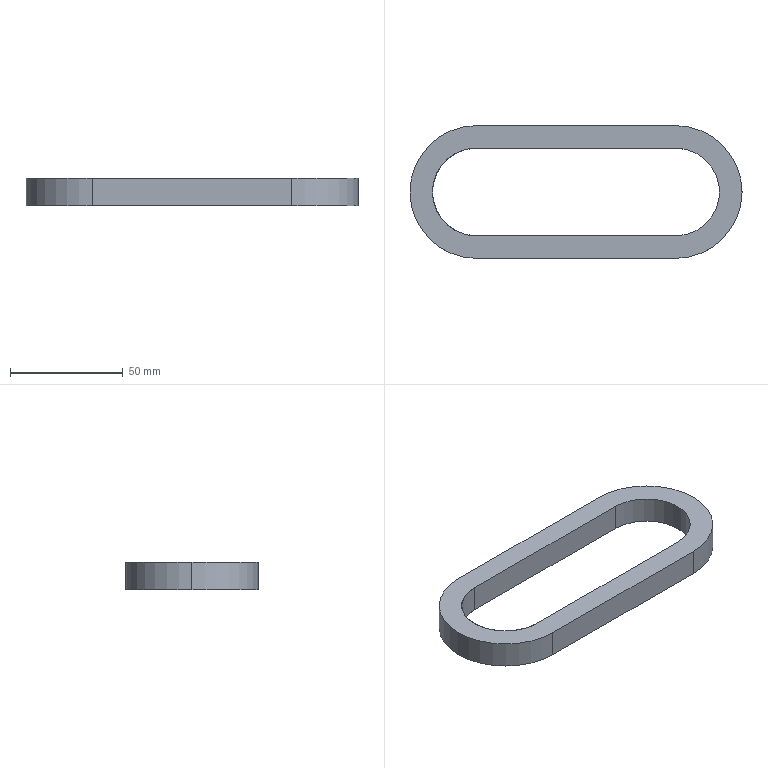Part | NX | features BREP 1, DATUM_CSYS 1, EXTRACT_DATUM_PLANE 1, EXTRUDE 1, SKETCH 1 | 2 solids | 22 faces | box 147.5 x 59 x 12 mm | volume 79425 mm3 | plane 12 | cylinder 10 | commonest cylinder face diameters 39 x5 59 x5
STEP:
#1=CARTESIAN_POINT('',(675.25,133.707,6.));
#2=VERTEX_POINT('',#1);
#3=CARTESIAN_POINT('',(675.25,133.707,-6.));
#4=VERTEX_POINT('',#3);
#5=CARTESIAN_POINT('',(675.25,133.707,6.));
#6=DIRECTION('',(0.,0.,-1.));
#7=VECTOR('',#6,1000.);
#8=LINE('',#5,#7);
#9=EDGE_CURVE('',#2,#4,#8,.T.);
#10=ORIENTED_EDGE('',*,*,#9,.F.);
#11=CARTESIAN_POINT('',(763.75,133.707,6.));
#12=VERTEX_POINT('',#11);
#13=CARTESIAN_POINT('',(675.25,133.707,6.));
#14=DIRECTION('',(1.,0.,0.));
#15=VECTOR('',#14,1000.);
#16=LINE('',#13,#15);
#17=EDGE_CURVE('',#2,#12,#16,.T.);
#18=ORIENTED_EDGE('',*,*,#17,.T.);
#19=CARTESIAN_POINT('',(763.75,133.707,-6.));
#20=VERTEX_POINT('',#19);
#21=CARTESIAN_POINT('',(763.75,133.707,-6.));
#22=DIRECTION('',(0.,0.,1.));
#23=VECTOR('',#22,1000.);
#24=LINE('',#21,#23);
#25=EDGE_CURVE('',#20,#12,#24,.T.);
#26=ORIENTED_EDGE('',*,*,#25,.F.);
#27=CARTESIAN_POINT('',(675.25,133.707,-6.));
#28=DIRECTION('',(1.,0.,0.));
#29=VECTOR('',#28,1000.);
#30=LINE('',#27,#29);
#31=EDGE_CURVE('',#4,#20,#30,.T.);
#32=ORIENTED_EDGE('',*,*,#31,.F.);
#33=EDGE_LOOP('',(#10,#18,#26,#32));
#34=FACE_BOUND('',#33,.T.);
#35=CARTESIAN_POINT('',(675.25,133.707,6.));
#36=DIRECTION('',(0.,-1.,0.));
#37=DIRECTION('',(0.,0.,1.));
#38=AXIS2_PLACEMENT_3D('',#35,#36,#37);
#39=PLANE('',#38);
#40=ADVANCED_FACE('',(#34),#39,.F.);
#41=ORIENTED_EDGE('',*,*,#31,.T.);
#42=CARTESIAN_POINT('',(763.75,74.707,-6.));
#43=VERTEX_POINT('',#42);
#44=CARTESIAN_POINT('',(763.75,104.207,-6.));
#45=DIRECTION('',(0.,0.,-1.));
#46=DIRECTION('',(0.,1.,0.));
#47=AXIS2_PLACEMENT_3D('',#44,#45,#46);
#48=CIRCLE('',#47,29.5);
#49=EDGE_CURVE('',#20,#43,#48,.T.);
#50=ORIENTED_EDGE('',*,*,#49,.T.);
#51=CARTESIAN_POINT('',(675.25,74.707,-6.));
#52=VERTEX_POINT('',#51);
#53=CARTESIAN_POINT('',(763.75,74.707,-6.));
#54=DIRECTION('',(-1.,0.,0.));
#55=VECTOR('',#54,1000.);
#56=LINE('',#53,#55);
#57=EDGE_CURVE('',#43,#52,#56,.T.);
#58=ORIENTED_EDGE('',*,*,#57,.T.);
#59=CARTESIAN_POINT('',(645.75,104.207,-6.));
#60=VERTEX_POINT('',#59);
#61=CARTESIAN_POINT('',(675.25,104.207,-6.));
#62=DIRECTION('',(0.,0.,-1.));
#63=DIRECTION('',(0.,-1.,0.));
#64=AXIS2_PLACEMENT_3D('',#61,#62,#63);
#65=CIRCLE('',#64,29.5);
#66=EDGE_CURVE('',#52,#60,#65,.T.);
#67=ORIENTED_EDGE('',*,*,#66,.T.);
#68=CARTESIAN_POINT('',(675.25,104.207,-6.));
#69=DIRECTION('',(0.,0.,-1.));
#70=DIRECTION('',(-1.,0.,0.));
#71=AXIS2_PLACEMENT_3D('',#68,#69,#70);
#72=CIRCLE('',#71,29.5);
#73=EDGE_CURVE('',#60,#4,#72,.T.);
#74=ORIENTED_EDGE('',*,*,#73,.T.);
#75=EDGE_LOOP('',(#41,#50,#58,#67,#74));
#76=FACE_BOUND('',#75,.T.);
#77=CARTESIAN_POINT('',(655.75,104.207,-6.));
#78=VERTEX_POINT('',#77);
#79=CARTESIAN_POINT('',(675.25,84.707,-6.));
#80=VERTEX_POINT('',#79);
#81=CARTESIAN_POINT('',(675.25,104.207,-6.));
#82=DIRECTION('',(0.,0.,1.));
#83=DIRECTION('',(-1.,0.,0.));
#84=AXIS2_PLACEMENT_3D('',#81,#82,#83);
#85=CIRCLE('',#84,19.5);
#86=EDGE_CURVE('',#78,#80,#85,.T.);
#87=ORIENTED_EDGE('',*,*,#86,.T.);
#88=CARTESIAN_POINT('',(763.75,84.707,-6.));
#89=VERTEX_POINT('',#88);
#90=CARTESIAN_POINT('',(763.75,84.707,-6.));
#91=DIRECTION('',(-1.,0.,0.));
#92=VECTOR('',#91,1000.);
#93=LINE('',#90,#92);
#94=EDGE_CURVE('',#89,#80,#93,.T.);
#95=ORIENTED_EDGE('',*,*,#94,.F.);
#96=CARTESIAN_POINT('',(763.75,123.707,-6.));
#97=VERTEX_POINT('',#96);
#98=CARTESIAN_POINT('',(763.75,104.207,-6.));
#99=DIRECTION('',(0.,0.,1.));
#100=DIRECTION('',(0.,-1.,0.));
#101=AXIS2_PLACEMENT_3D('',#98,#99,#100);
#102=CIRCLE('',#101,19.5);
#103=EDGE_CURVE('',#89,#97,#102,.T.);
#104=ORIENTED_EDGE('',*,*,#103,.T.);
#105=CARTESIAN_POINT('',(675.25,123.707,-6.));
#106=VERTEX_POINT('',#105);
#107=CARTESIAN_POINT('',(675.25,123.707,-6.));
#108=DIRECTION('',(1.,0.,0.));
#109=VECTOR('',#108,1000.);
#110=LINE('',#107,#109);
#111=EDGE_CURVE('',#106,#97,#110,.T.);
#112=ORIENTED_EDGE('',*,*,#111,.F.);
#113=CARTESIAN_POINT('',(675.25,104.207,-6.));
#114=DIRECTION('',(0.,0.,1.));
#115=DIRECTION('',(0.,1.,0.));
#116=AXIS2_PLACEMENT_3D('',#113,#114,#115);
#117=CIRCLE('',#116,19.5);
#118=EDGE_CURVE('',#106,#78,#117,.T.);
#119=ORIENTED_EDGE('',*,*,#118,.T.);
#120=EDGE_LOOP('',(#87,#95,#104,#112,#119));
#121=FACE_BOUND('',#120,.T.);
#122=CARTESIAN_POINT('',(675.25,104.207,-6.));
#123=DIRECTION('',(0.,0.,1.));
#124=DIRECTION('',(-1.,0.,0.));
#125=AXIS2_PLACEMENT_3D('',#122,#123,#124);
#126=PLANE('',#125);
#127=ADVANCED_FACE('',(#76,#121),#126,.F.);
#128=CARTESIAN_POINT('',(645.75,104.207,6.));
#129=VERTEX_POINT('',#128);
#130=CARTESIAN_POINT('',(675.25,104.207,6.));
#131=DIRECTION('',(0.,0.,1.));
#132=DIRECTION('',(0.,1.,0.));
#133=AXIS2_PLACEMENT_3D('',#130,#131,#132);
#134=CIRCLE('',#133,29.5);
#135=EDGE_CURVE('',#2,#129,#134,.T.);
#136=ORIENTED_EDGE('',*,*,#135,.F.);
#137=ORIENTED_EDGE('',*,*,#9,.T.);
#138=ORIENTED_EDGE('',*,*,#73,.F.);
#139=CARTESIAN_POINT('',(645.75,104.207,-6.));
#140=DIRECTION('',(0.,0.,1.));
#141=VECTOR('',#140,1000.);
#142=LINE('',#139,#141);
#143=EDGE_CURVE('',#60,#129,#142,.T.);
#144=ORIENTED_EDGE('',*,*,#143,.T.);
#145=EDGE_LOOP('',(#136,#137,#138,#144));
#146=FACE_BOUND('',#145,.T.);
#147=CARTESIAN_POINT('',(675.25,104.207,6.));
#148=DIRECTION('',(0.,0.,-1.));
#149=DIRECTION('',(1.,0.,0.));
#150=AXIS2_PLACEMENT_3D('',#147,#148,#149);
#151=CYLINDRICAL_SURFACE('',#150,29.5);
#152=ADVANCED_FACE('',(#146),#151,.T.);
#153=ORIENTED_EDGE('',*,*,#143,.F.);
#154=ORIENTED_EDGE('',*,*,#66,.F.);
#155=CARTESIAN_POINT('',(675.25,74.707,6.));
#156=VERTEX_POINT('',#155);
#157=CARTESIAN_POINT('',(675.25,74.707,-6.));
#158=DIRECTION('',(0.,0.,1.));
#159=VECTOR('',#158,1000.);
#160=LINE('',#157,#159);
#161=EDGE_CURVE('',#52,#156,#160,.T.);
#162=ORIENTED_EDGE('',*,*,#161,.T.);
#163=CARTESIAN_POINT('',(675.25,104.207,6.));
#164=DIRECTION('',(0.,0.,1.));
#165=DIRECTION('',(-1.,0.,0.));
#166=AXIS2_PLACEMENT_3D('',#163,#164,#165);
#167=CIRCLE('',#166,29.5);
#168=EDGE_CURVE('',#129,#156,#167,.T.);
#169=ORIENTED_EDGE('',*,*,#168,.F.);
#170=EDGE_LOOP('',(#153,#154,#162,#169));
#171=FACE_BOUND('',#170,.T.);
#172=CARTESIAN_POINT('',(675.25,104.207,6.));
#173=DIRECTION('',(0.,0.,-1.));
#174=DIRECTION('',(1.,0.,0.));
#175=AXIS2_PLACEMENT_3D('',#172,#173,#174);
#176=CYLINDRICAL_SURFACE('',#175,29.5);
#177=ADVANCED_FACE('',(#171),#176,.T.);
#178=ORIENTED_EDGE('',*,*,#168,.T.);
#179=CARTESIAN_POINT('',(763.75,74.707,6.));
#180=VERTEX_POINT('',#179);
#181=CARTESIAN_POINT('',(763.75,74.707,6.));
#182=DIRECTION('',(-1.,0.,0.));
#183=VECTOR('',#182,1000.);
#184=LINE('',#181,#183);
#185=EDGE_CURVE('',#180,#156,#184,.T.);
#186=ORIENTED_EDGE('',*,*,#185,.F.);
#187=CARTESIAN_POINT('',(763.75,104.207,6.));
#188=DIRECTION('',(0.,0.,1.));
#189=DIRECTION('',(0.,-1.,0.));
#190=AXIS2_PLACEMENT_3D('',#187,#188,#189);
#191=CIRCLE('',#190,29.5);
#192=EDGE_CURVE('',#180,#12,#191,.T.);
#193=ORIENTED_EDGE('',*,*,#192,.T.);
#194=ORIENTED_EDGE('',*,*,#17,.F.);
#195=ORIENTED_EDGE('',*,*,#135,.T.);
#196=EDGE_LOOP('',(#178,#186,#193,#194,#195));
#197=FACE_BOUND('',#196,.T.);
#198=CARTESIAN_POINT('',(675.25,84.707,6.));
#199=VERTEX_POINT('',#198);
#200=CARTESIAN_POINT('',(655.75,104.207,6.));
#201=VERTEX_POINT('',#200);
#202=CARTESIAN_POINT('',(675.25,104.207,6.));
#203=DIRECTION('',(0.,0.,-1.));
#204=DIRECTION('',(0.,-1.,0.));
#205=AXIS2_PLACEMENT_3D('',#202,#203,#204);
#206=CIRCLE('',#205,19.5);
#207=EDGE_CURVE('',#199,#201,#206,.T.);
#208=ORIENTED_EDGE('',*,*,#207,.T.);
#209=CARTESIAN_POINT('',(675.25,123.707,6.));
#210=VERTEX_POINT('',#209);
#211=CARTESIAN_POINT('',(675.25,104.207,6.));
#212=DIRECTION('',(0.,0.,-1.));
#213=DIRECTION('',(-1.,0.,0.));
#214=AXIS2_PLACEMENT_3D('',#211,#212,#213);
#215=CIRCLE('',#214,19.5);
#216=EDGE_CURVE('',#201,#210,#215,.T.);
#217=ORIENTED_EDGE('',*,*,#216,.T.);
#218=CARTESIAN_POINT('',(763.75,123.707,6.));
#219=VERTEX_POINT('',#218);
#220=CARTESIAN_POINT('',(675.25,123.707,6.));
#221=DIRECTION('',(1.,0.,0.));
#222=VECTOR('',#221,1000.);
#223=LINE('',#220,#222);
#224=EDGE_CURVE('',#210,#219,#223,.T.);
#225=ORIENTED_EDGE('',*,*,#224,.T.);
#226=CARTESIAN_POINT('',(763.75,84.707,6.));
#227=VERTEX_POINT('',#226);
#228=CARTESIAN_POINT('',(763.75,104.207,6.));
#229=DIRECTION('',(0.,0.,-1.));
#230=DIRECTION('',(0.,1.,0.));
#231=AXIS2_PLACEMENT_3D('',#228,#229,#230);
#232=CIRCLE('',#231,19.5);
#233=EDGE_CURVE('',#219,#227,#232,.T.);
#234=ORIENTED_EDGE('',*,*,#233,.T.);
#235=CARTESIAN_POINT('',(763.75,84.707,6.));
#236=DIRECTION('',(-1.,0.,0.));
#237=VECTOR('',#236,1000.);
#238=LINE('',#235,#237);
#239=EDGE_CURVE('',#227,#199,#238,.T.);
#240=ORIENTED_EDGE('',*,*,#239,.T.);
#241=EDGE_LOOP('',(#208,#217,#225,#234,#240));
#242=FACE_BOUND('',#241,.T.);
#243=CARTESIAN_POINT('',(675.25,104.207,6.));
#244=DIRECTION('',(0.,0.,1.));
#245=DIRECTION('',(-1.,0.,0.));
#246=AXIS2_PLACEMENT_3D('',#243,#244,#245);
#247=PLANE('',#246);
#248=ADVANCED_FACE('',(#197,#242),#247,.T.);
#249=ORIENTED_EDGE('',*,*,#25,.T.);
#250=ORIENTED_EDGE('',*,*,#192,.F.);
#251=CARTESIAN_POINT('',(763.75,74.707,6.));
#252=DIRECTION('',(0.,0.,-1.));
#253=VECTOR('',#252,1000.);
#254=LINE('',#251,#253);
#255=EDGE_CURVE('',#180,#43,#254,.T.);
#256=ORIENTED_EDGE('',*,*,#255,.T.);
#257=ORIENTED_EDGE('',*,*,#49,.F.);
#258=EDGE_LOOP('',(#249,#250,#256,#257));
#259=FACE_BOUND('',#258,.T.);
#260=CARTESIAN_POINT('',(763.75,104.207,6.));
#261=DIRECTION('',(0.,0.,-1.));
#262=DIRECTION('',(1.,0.,0.));
#263=AXIS2_PLACEMENT_3D('',#260,#261,#262);
#264=CYLINDRICAL_SURFACE('',#263,29.5);
#265=ADVANCED_FACE('',(#259),#264,.T.);
#266=ORIENTED_EDGE('',*,*,#255,.F.);
#267=ORIENTED_EDGE('',*,*,#185,.T.);
#268=ORIENTED_EDGE('',*,*,#161,.F.);
#269=ORIENTED_EDGE('',*,*,#57,.F.);
#270=EDGE_LOOP('',(#266,#267,#268,#269));
#271=FACE_BOUND('',#270,.T.);
#272=CARTESIAN_POINT('',(675.25,74.707,6.));
#273=DIRECTION('',(0.,1.,0.));
#274=DIRECTION('',(1.,0.,0.));
#275=AXIS2_PLACEMENT_3D('',#272,#273,#274);
#276=PLANE('',#275);
#277=ADVANCED_FACE('',(#271),#276,.F.);
#278=CARTESIAN_POINT('',(675.25,84.707,6.));
#279=DIRECTION('',(0.,0.,-1.));
#280=VECTOR('',#279,1000.);
#281=LINE('',#278,#280);
#282=EDGE_CURVE('',#199,#80,#281,.T.);
#283=ORIENTED_EDGE('',*,*,#282,.F.);
#284=ORIENTED_EDGE('',*,*,#239,.F.);
#285=CARTESIAN_POINT('',(763.75,84.707,-6.));
#286=DIRECTION('',(0.,0.,1.));
#287=VECTOR('',#286,1000.);
#288=LINE('',#285,#287);
#289=EDGE_CURVE('',#89,#227,#288,.T.);
#290=ORIENTED_EDGE('',*,*,#289,.F.);
#291=ORIENTED_EDGE('',*,*,#94,.T.);
#292=EDGE_LOOP('',(#283,#284,#290,#291));
#293=FACE_BOUND('',#292,.T.);
#294=CARTESIAN_POINT('',(675.25,84.707,6.));
#295=DIRECTION('',(0.,1.,0.));
#296=DIRECTION('',(1.,0.,0.));
#297=AXIS2_PLACEMENT_3D('',#294,#295,#296);
#298=PLANE('',#297);
#299=ADVANCED_FACE('',(#293),#298,.T.);
#300=ORIENTED_EDGE('',*,*,#289,.T.);
#301=ORIENTED_EDGE('',*,*,#233,.F.);
#302=CARTESIAN_POINT('',(763.75,123.707,6.));
#303=DIRECTION('',(0.,0.,-1.));
#304=VECTOR('',#303,1000.);
#305=LINE('',#302,#304);
#306=EDGE_CURVE('',#219,#97,#305,.T.);
#307=ORIENTED_EDGE('',*,*,#306,.T.);
#308=ORIENTED_EDGE('',*,*,#103,.F.);
#309=EDGE_LOOP('',(#300,#301,#307,#308));
#310=FACE_BOUND('',#309,.T.);
#311=CARTESIAN_POINT('',(763.75,104.207,6.));
#312=DIRECTION('',(0.,0.,-1.));
#313=DIRECTION('',(1.,0.,0.));
#314=AXIS2_PLACEMENT_3D('',#311,#312,#313);
#315=CYLINDRICAL_SURFACE('',#314,19.5);
#316=ADVANCED_FACE('',(#310),#315,.F.);
#317=ORIENTED_EDGE('',*,*,#306,.F.);
#318=ORIENTED_EDGE('',*,*,#224,.F.);
#319=CARTESIAN_POINT('',(675.25,123.707,-6.));
#320=DIRECTION('',(0.,0.,1.));
#321=VECTOR('',#320,1000.);
#322=LINE('',#319,#321);
#323=EDGE_CURVE('',#106,#210,#322,.T.);
#324=ORIENTED_EDGE('',*,*,#323,.F.);
#325=ORIENTED_EDGE('',*,*,#111,.T.);
#326=EDGE_LOOP('',(#317,#318,#324,#325));
#327=FACE_BOUND('',#326,.T.);
#328=CARTESIAN_POINT('',(675.25,123.707,6.));
#329=DIRECTION('',(0.,-1.,0.));
#330=DIRECTION('',(0.,0.,1.));
#331=AXIS2_PLACEMENT_3D('',#328,#329,#330);
#332=PLANE('',#331);
#333=ADVANCED_FACE('',(#327),#332,.T.);
#334=CARTESIAN_POINT('',(655.75,104.207,-6.));
#335=DIRECTION('',(0.,0.,1.));
#336=VECTOR('',#335,1000.);
#337=LINE('',#334,#336);
#338=EDGE_CURVE('',#78,#201,#337,.T.);
#339=ORIENTED_EDGE('',*,*,#338,.F.);
#340=ORIENTED_EDGE('',*,*,#118,.F.);
#341=ORIENTED_EDGE('',*,*,#323,.T.);
#342=ORIENTED_EDGE('',*,*,#216,.F.);
#343=EDGE_LOOP('',(#339,#340,#341,#342));
#344=FACE_BOUND('',#343,.T.);
#345=CARTESIAN_POINT('',(675.25,104.207,6.));
#346=DIRECTION('',(0.,0.,-1.));
#347=DIRECTION('',(1.,0.,0.));
#348=AXIS2_PLACEMENT_3D('',#345,#346,#347);
#349=CYLINDRICAL_SURFACE('',#348,19.5);
#350=ADVANCED_FACE('',(#344),#349,.F.);
#351=ORIENTED_EDGE('',*,*,#207,.F.);
#352=ORIENTED_EDGE('',*,*,#282,.T.);
#353=ORIENTED_EDGE('',*,*,#86,.F.);
#354=ORIENTED_EDGE('',*,*,#338,.T.);
#355=EDGE_LOOP('',(#351,#352,#353,#354));
#356=FACE_BOUND('',#355,.T.);
#357=CARTESIAN_POINT('',(675.25,104.207,6.));
#358=DIRECTION('',(0.,0.,-1.));
#359=DIRECTION('',(1.,0.,0.));
#360=AXIS2_PLACEMENT_3D('',#357,#358,#359);
#361=CYLINDRICAL_SURFACE('',#360,19.5);
#362=ADVANCED_FACE('',(#356),#361,.F.);
#363=CLOSED_SHELL('',(#40,#127,#152,#177,#248,#265,#277,#299,#316,#333,#350,#362));
#364=MANIFOLD_SOLID_BREP('',#363);
#365=CARTESIAN_POINT('',(675.25,84.707,-6.));
#366=VERTEX_POINT('',#365);
#367=CARTESIAN_POINT('',(675.25,123.707,-6.));
#368=VERTEX_POINT('',#367);
#369=CARTESIAN_POINT('',(675.25,104.207,-6.));
#370=DIRECTION('',(0.,0.,-1.));
#371=DIRECTION('',(-1.,0.,0.));
#372=AXIS2_PLACEMENT_3D('',#369,#370,#371);
#373=CIRCLE('',#372,19.5);
#374=EDGE_CURVE('',#366,#368,#373,.T.);
#375=ORIENTED_EDGE('',*,*,#374,.T.);
#376=CARTESIAN_POINT('',(675.25,123.707,6.));
#377=VERTEX_POINT('',#376);
#378=CARTESIAN_POINT('',(675.25,123.707,6.));
#379=DIRECTION('',(0.,0.,-1.));
#380=VECTOR('',#379,1000.);
#381=LINE('',#378,#380);
#382=EDGE_CURVE('',#377,#368,#381,.T.);
#383=ORIENTED_EDGE('',*,*,#382,.F.);
#384=CARTESIAN_POINT('',(675.25,84.707,6.));
#385=VERTEX_POINT('',#384);
#386=CARTESIAN_POINT('',(675.25,104.207,6.));
#387=DIRECTION('',(0.,0.,-1.));
#388=DIRECTION('',(0.,-1.,0.));
#389=AXIS2_PLACEMENT_3D('',#386,#387,#388);
#390=CIRCLE('',#389,19.5);
#391=EDGE_CURVE('',#385,#377,#390,.T.);
#392=ORIENTED_EDGE('',*,*,#391,.F.);
#393=CARTESIAN_POINT('',(675.25,84.707,6.));
#394=DIRECTION('',(0.,0.,-1.));
#395=VECTOR('',#394,1000.);
#396=LINE('',#393,#395);
#397=EDGE_CURVE('',#385,#366,#396,.T.);
#398=ORIENTED_EDGE('',*,*,#397,.T.);
#399=EDGE_LOOP('',(#375,#383,#392,#398));
#400=FACE_BOUND('',#399,.T.);
#401=CARTESIAN_POINT('',(675.25,104.207,6.));
#402=DIRECTION('',(0.,0.,-1.));
#403=DIRECTION('',(-1.,0.,0.));
#404=AXIS2_PLACEMENT_3D('',#401,#402,#403);
#405=CYLINDRICAL_SURFACE('',#404,19.5);
#406=ADVANCED_FACE('',(#400),#405,.F.);
#407=CARTESIAN_POINT('',(763.75,123.707,-6.));
#408=VERTEX_POINT('',#407);
#409=CARTESIAN_POINT('',(675.25,123.707,-6.));
#410=DIRECTION('',(1.,0.,0.));
#411=VECTOR('',#410,1000.);
#412=LINE('',#409,#411);
#413=EDGE_CURVE('',#368,#408,#412,.T.);
#414=ORIENTED_EDGE('',*,*,#413,.T.);
#415=CARTESIAN_POINT('',(763.75,123.707,6.));
#416=VERTEX_POINT('',#415);
#417=CARTESIAN_POINT('',(763.75,123.707,6.));
#418=DIRECTION('',(0.,0.,-1.));
#419=VECTOR('',#418,1000.);
#420=LINE('',#417,#419);
#421=EDGE_CURVE('',#416,#408,#420,.T.);
#422=ORIENTED_EDGE('',*,*,#421,.F.);
#423=CARTESIAN_POINT('',(675.25,123.707,6.));
#424=DIRECTION('',(1.,0.,0.));
#425=VECTOR('',#424,1000.);
#426=LINE('',#423,#425);
#427=EDGE_CURVE('',#377,#416,#426,.T.);
#428=ORIENTED_EDGE('',*,*,#427,.F.);
#429=ORIENTED_EDGE('',*,*,#382,.T.);
#430=EDGE_LOOP('',(#414,#422,#428,#429));
#431=FACE_BOUND('',#430,.T.);
#432=CARTESIAN_POINT('',(675.25,123.707,6.));
#433=DIRECTION('',(0.,1.,0.));
#434=DIRECTION('',(0.,0.,1.));
#435=AXIS2_PLACEMENT_3D('',#432,#433,#434);
#436=PLANE('',#435);
#437=ADVANCED_FACE('',(#431),#436,.F.);
#438=CARTESIAN_POINT('',(763.75,84.707,-6.));
#439=VERTEX_POINT('',#438);
#440=CARTESIAN_POINT('',(763.75,104.207,-6.));
#441=DIRECTION('',(0.,0.,-1.));
#442=DIRECTION('',(0.,1.,0.));
#443=AXIS2_PLACEMENT_3D('',#440,#441,#442);
#444=CIRCLE('',#443,19.5);
#445=EDGE_CURVE('',#408,#439,#444,.T.);
#446=ORIENTED_EDGE('',*,*,#445,.T.);
#447=CARTESIAN_POINT('',(763.75,84.707,6.));
#448=VERTEX_POINT('',#447);
#449=CARTESIAN_POINT('',(763.75,84.707,6.));
#450=DIRECTION('',(0.,0.,-1.));
#451=VECTOR('',#450,1000.);
#452=LINE('',#449,#451);
#453=EDGE_CURVE('',#448,#439,#452,.T.);
#454=ORIENTED_EDGE('',*,*,#453,.F.);
#455=CARTESIAN_POINT('',(763.75,104.207,6.));
#456=DIRECTION('',(0.,0.,-1.));
#457=DIRECTION('',(0.,1.,0.));
#458=AXIS2_PLACEMENT_3D('',#455,#456,#457);
#459=CIRCLE('',#458,19.5);
#460=EDGE_CURVE('',#416,#448,#459,.T.);
#461=ORIENTED_EDGE('',*,*,#460,.F.);
#462=ORIENTED_EDGE('',*,*,#421,.T.);
#463=EDGE_LOOP('',(#446,#454,#461,#462));
#464=FACE_BOUND('',#463,.T.);
#465=CARTESIAN_POINT('',(763.75,104.207,6.));
#466=DIRECTION('',(0.,0.,-1.));
#467=DIRECTION('',(-1.,0.,0.));
#468=AXIS2_PLACEMENT_3D('',#465,#466,#467);
#469=CYLINDRICAL_SURFACE('',#468,19.5);
#470=ADVANCED_FACE('',(#464),#469,.F.);
#471=CARTESIAN_POINT('',(675.25,133.707,-6.));
#472=VERTEX_POINT('',#471);
#473=CARTESIAN_POINT('',(675.25,74.707,-6.));
#474=VERTEX_POINT('',#473);
#475=CARTESIAN_POINT('',(675.25,104.207,-6.));
#476=DIRECTION('',(0.,0.,1.));
#477=DIRECTION('',(-1.,0.,0.));
#478=AXIS2_PLACEMENT_3D('',#475,#476,#477);
#479=CIRCLE('',#478,29.5);
#480=EDGE_CURVE('',#472,#474,#479,.T.);
#481=ORIENTED_EDGE('',*,*,#480,.T.);
#482=CARTESIAN_POINT('',(675.25,74.707,6.));
#483=VERTEX_POINT('',#482);
#484=CARTESIAN_POINT('',(675.25,74.707,6.));
#485=DIRECTION('',(0.,0.,-1.));
#486=VECTOR('',#485,1000.);
#487=LINE('',#484,#486);
#488=EDGE_CURVE('',#483,#474,#487,.T.);
#489=ORIENTED_EDGE('',*,*,#488,.F.);
#490=CARTESIAN_POINT('',(675.25,133.707,6.));
#491=VERTEX_POINT('',#490);
#492=CARTESIAN_POINT('',(675.25,104.207,6.));
#493=DIRECTION('',(0.,0.,1.));
#494=DIRECTION('',(0.,1.,0.));
#495=AXIS2_PLACEMENT_3D('',#492,#493,#494);
#496=CIRCLE('',#495,29.5);
#497=EDGE_CURVE('',#491,#483,#496,.T.);
#498=ORIENTED_EDGE('',*,*,#497,.F.);
#499=CARTESIAN_POINT('',(675.25,133.707,6.));
#500=DIRECTION('',(0.,0.,-1.));
#501=VECTOR('',#500,1000.);
#502=LINE('',#499,#501);
#503=EDGE_CURVE('',#491,#472,#502,.T.);
#504=ORIENTED_EDGE('',*,*,#503,.T.);
#505=EDGE_LOOP('',(#481,#489,#498,#504));
#506=FACE_BOUND('',#505,.T.);
#507=CARTESIAN_POINT('',(675.25,104.207,6.));
#508=DIRECTION('',(0.,0.,-1.));
#509=DIRECTION('',(-1.,0.,0.));
#510=AXIS2_PLACEMENT_3D('',#507,#508,#509);
#511=CYLINDRICAL_SURFACE('',#510,29.5);
#512=ADVANCED_FACE('',(#506),#511,.T.);
#513=CARTESIAN_POINT('',(763.75,74.707,-6.));
#514=VERTEX_POINT('',#513);
#515=CARTESIAN_POINT('',(675.25,74.707,-6.));
#516=DIRECTION('',(1.,0.,0.));
#517=VECTOR('',#516,1000.);
#518=LINE('',#515,#517);
#519=EDGE_CURVE('',#474,#514,#518,.T.);
#520=ORIENTED_EDGE('',*,*,#519,.T.);
#521=CARTESIAN_POINT('',(763.75,74.707,6.));
#522=VERTEX_POINT('',#521);
#523=CARTESIAN_POINT('',(763.75,74.707,6.));
#524=DIRECTION('',(0.,0.,-1.));
#525=VECTOR('',#524,1000.);
#526=LINE('',#523,#525);
#527=EDGE_CURVE('',#522,#514,#526,.T.);
#528=ORIENTED_EDGE('',*,*,#527,.F.);
#529=CARTESIAN_POINT('',(675.25,74.707,6.));
#530=DIRECTION('',(1.,0.,0.));
#531=VECTOR('',#530,1000.);
#532=LINE('',#529,#531);
#533=EDGE_CURVE('',#483,#522,#532,.T.);
#534=ORIENTED_EDGE('',*,*,#533,.F.);
#535=ORIENTED_EDGE('',*,*,#488,.T.);
#536=EDGE_LOOP('',(#520,#528,#534,#535));
#537=FACE_BOUND('',#536,.T.);
#538=CARTESIAN_POINT('',(675.25,74.707,6.));
#539=DIRECTION('',(0.,1.,0.));
#540=DIRECTION('',(0.,0.,1.));
#541=AXIS2_PLACEMENT_3D('',#538,#539,#540);
#542=PLANE('',#541);
#543=ADVANCED_FACE('',(#537),#542,.F.);
#544=CARTESIAN_POINT('',(763.75,133.707,-6.));
#545=VERTEX_POINT('',#544);
#546=CARTESIAN_POINT('',(763.75,104.207,-6.));
#547=DIRECTION('',(0.,0.,1.));
#548=DIRECTION('',(0.,-1.,0.));
#549=AXIS2_PLACEMENT_3D('',#546,#547,#548);
#550=CIRCLE('',#549,29.5);
#551=EDGE_CURVE('',#514,#545,#550,.T.);
#552=ORIENTED_EDGE('',*,*,#551,.T.);
#553=CARTESIAN_POINT('',(763.75,133.707,6.));
#554=VERTEX_POINT('',#553);
#555=CARTESIAN_POINT('',(763.75,133.707,6.));
#556=DIRECTION('',(0.,0.,-1.));
#557=VECTOR('',#556,1000.);
#558=LINE('',#555,#557);
#559=EDGE_CURVE('',#554,#545,#558,.T.);
#560=ORIENTED_EDGE('',*,*,#559,.F.);
#561=CARTESIAN_POINT('',(763.75,104.207,6.));
#562=DIRECTION('',(0.,0.,1.));
#563=DIRECTION('',(0.,-1.,0.));
#564=AXIS2_PLACEMENT_3D('',#561,#562,#563);
#565=CIRCLE('',#564,29.5);
#566=EDGE_CURVE('',#522,#554,#565,.T.);
#567=ORIENTED_EDGE('',*,*,#566,.F.);
#568=ORIENTED_EDGE('',*,*,#527,.T.);
#569=EDGE_LOOP('',(#552,#560,#567,#568));
#570=FACE_BOUND('',#569,.T.);
#571=CARTESIAN_POINT('',(763.75,104.207,6.));
#572=DIRECTION('',(0.,0.,-1.));
#573=DIRECTION('',(-1.,0.,0.));
#574=AXIS2_PLACEMENT_3D('',#571,#572,#573);
#575=CYLINDRICAL_SURFACE('',#574,29.5);
#576=ADVANCED_FACE('',(#570),#575,.T.);
#577=CARTESIAN_POINT('',(763.75,133.707,-6.));
#578=DIRECTION('',(-1.,0.,0.));
#579=VECTOR('',#578,1000.);
#580=LINE('',#577,#579);
#581=EDGE_CURVE('',#545,#472,#580,.T.);
#582=ORIENTED_EDGE('',*,*,#581,.T.);
#583=ORIENTED_EDGE('',*,*,#503,.F.);
#584=CARTESIAN_POINT('',(763.75,133.707,6.));
#585=DIRECTION('',(-1.,0.,0.));
#586=VECTOR('',#585,1000.);
#587=LINE('',#584,#586);
#588=EDGE_CURVE('',#554,#491,#587,.T.);
#589=ORIENTED_EDGE('',*,*,#588,.F.);
#590=ORIENTED_EDGE('',*,*,#559,.T.);
#591=EDGE_LOOP('',(#582,#583,#589,#590));
#592=FACE_BOUND('',#591,.T.);
#593=CARTESIAN_POINT('',(763.75,133.707,6.));
#594=DIRECTION('',(0.,-1.,0.));
#595=DIRECTION('',(0.,0.,-1.));
#596=AXIS2_PLACEMENT_3D('',#593,#594,#595);
#597=PLANE('',#596);
#598=ADVANCED_FACE('',(#592),#597,.F.);
#599=CARTESIAN_POINT('',(763.75,84.707,-6.));
#600=DIRECTION('',(-1.,0.,0.));
#601=VECTOR('',#600,1000.);
#602=LINE('',#599,#601);
#603=EDGE_CURVE('',#439,#366,#602,.T.);
#604=ORIENTED_EDGE('',*,*,#603,.T.);
#605=ORIENTED_EDGE('',*,*,#397,.F.);
#606=CARTESIAN_POINT('',(763.75,84.707,6.));
#607=DIRECTION('',(-1.,0.,0.));
#608=VECTOR('',#607,1000.);
#609=LINE('',#606,#608);
#610=EDGE_CURVE('',#448,#385,#609,.T.);
#611=ORIENTED_EDGE('',*,*,#610,.F.);
#612=ORIENTED_EDGE('',*,*,#453,.T.);
#613=EDGE_LOOP('',(#604,#605,#611,#612));
#614=FACE_BOUND('',#613,.T.);
#615=CARTESIAN_POINT('',(763.75,84.707,6.));
#616=DIRECTION('',(0.,-1.,0.));
#617=DIRECTION('',(0.,0.,-1.));
#618=AXIS2_PLACEMENT_3D('',#615,#616,#617);
#619=PLANE('',#618);
#620=ADVANCED_FACE('',(#614),#619,.F.);
#621=ORIENTED_EDGE('',*,*,#497,.T.);
#622=ORIENTED_EDGE('',*,*,#533,.T.);
#623=ORIENTED_EDGE('',*,*,#566,.T.);
#624=ORIENTED_EDGE('',*,*,#588,.T.);
#625=EDGE_LOOP('',(#621,#622,#623,#624));
#626=FACE_BOUND('',#625,.T.);
#627=ORIENTED_EDGE('',*,*,#391,.T.);
#628=ORIENTED_EDGE('',*,*,#427,.T.);
#629=ORIENTED_EDGE('',*,*,#460,.T.);
#630=ORIENTED_EDGE('',*,*,#610,.T.);
#631=EDGE_LOOP('',(#627,#628,#629,#630));
#632=FACE_BOUND('',#631,.T.);
#633=CARTESIAN_POINT('',(675.25,104.207,6.));
#634=DIRECTION('',(0.,0.,1.));
#635=DIRECTION('',(1.,0.,0.));
#636=AXIS2_PLACEMENT_3D('',#633,#634,#635);
#637=PLANE('',#636);
#638=ADVANCED_FACE('',(#626,#632),#637,.T.);
#639=ORIENTED_EDGE('',*,*,#480,.F.);
#640=ORIENTED_EDGE('',*,*,#581,.F.);
#641=ORIENTED_EDGE('',*,*,#551,.F.);
#642=ORIENTED_EDGE('',*,*,#519,.F.);
#643=EDGE_LOOP('',(#639,#640,#641,#642));
#644=FACE_BOUND('',#643,.T.);
#645=ORIENTED_EDGE('',*,*,#374,.F.);
#646=ORIENTED_EDGE('',*,*,#603,.F.);
#647=ORIENTED_EDGE('',*,*,#445,.F.);
#648=ORIENTED_EDGE('',*,*,#413,.F.);
#649=EDGE_LOOP('',(#645,#646,#647,#648));
#650=FACE_BOUND('',#649,.T.);
#651=CARTESIAN_POINT('',(675.25,104.207,-6.));
#652=DIRECTION('',(0.,0.,1.));
#653=DIRECTION('',(1.,0.,0.));
#654=AXIS2_PLACEMENT_3D('',#651,#652,#653);
#655=PLANE('',#654);
#656=ADVANCED_FACE('',(#644,#650),#655,.F.);
#657=CLOSED_SHELL('',(#406,#437,#470,#512,#543,#576,#598,#620,#638,#656));
#658=MANIFOLD_SOLID_BREP('',#657);
#659=(LENGTH_UNIT()NAMED_UNIT(*)SI_UNIT(.MILLI.,.METRE.));
#660=UNCERTAINTY_MEASURE_WITH_UNIT(LENGTH_MEASURE(0.00001),#659,'','');
#661=(NAMED_UNIT(*)PLANE_ANGLE_UNIT()SI_UNIT($,.RADIAN.));
#662=(NAMED_UNIT(*)SI_UNIT($,.STERADIAN.)SOLID_ANGLE_UNIT());
#663=(GEOMETRIC_REPRESENTATION_CONTEXT(3)GLOBAL_UNCERTAINTY_ASSIGNED_CONTEXT((#660))GLOBAL_UNIT_ASSIGNED_CONTEXT((#659,#661,#662))REPRESENTATION_CONTEXT('',''));
#664=ADVANCED_BREP_SHAPE_REPRESENTATION('',(#364,#658),#663);